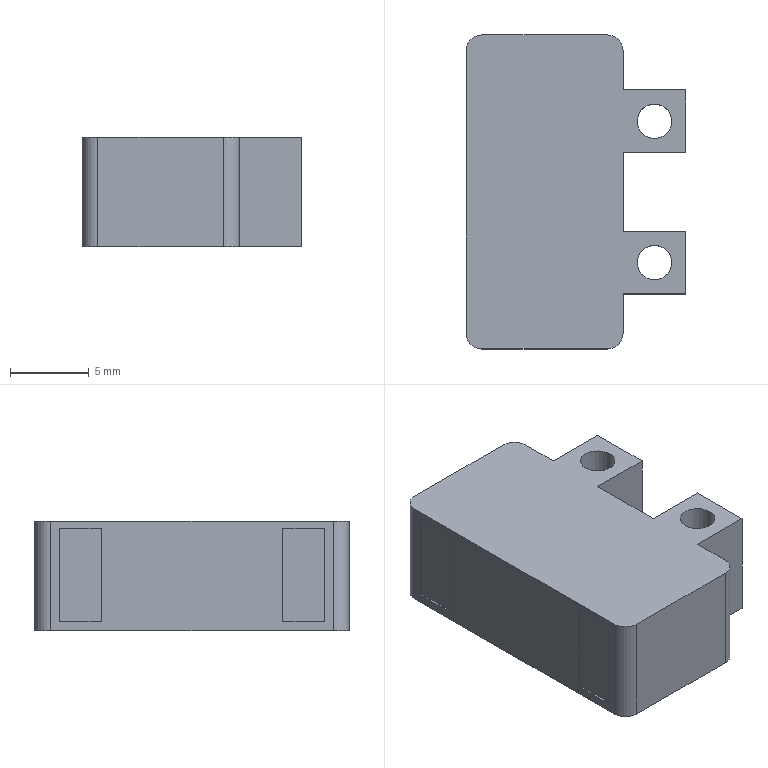Part | SolidWorks | features ICE 2, Extrusion 1, Fillet 1, MirrorPattern 1 | 1 solid | 32 faces | box 14 x 20 x 7 mm | volume 1562 mm3 | plane 24 | cylinder 8 | commonest cylinder face diameters 2 x4 2.2 x4
STEP:
#1=CARTESIAN_POINT('',(5.9,-4.5,0.));
#2=VERTEX_POINT('',#1);
#3=CARTESIAN_POINT('',(8.1,-4.5,0.));
#4=VERTEX_POINT('',#3);
#5=CARTESIAN_POINT('',(7.,-4.5,0.));
#6=DIRECTION('',(0.,0.,1.));
#7=DIRECTION('',(1.,0.,0.));
#8=AXIS2_PLACEMENT_3D('',#5,#6,#7);
#9=CIRCLE('',#8,1.1);
#10=EDGE_CURVE('',#2,#4,#9,.T.);
#11=ORIENTED_EDGE('',*,*,#10,.F.);
#12=CARTESIAN_POINT('',(5.9,-4.5,7.));
#13=VERTEX_POINT('',#12);
#14=CARTESIAN_POINT('',(5.9,-4.5,0.));
#15=DIRECTION('',(0.,0.,1.));
#16=VECTOR('',#15,1000.);
#17=LINE('',#14,#16);
#18=EDGE_CURVE('',#2,#13,#17,.T.);
#19=ORIENTED_EDGE('',*,*,#18,.T.);
#20=CARTESIAN_POINT('',(8.1,-4.5,7.));
#21=VERTEX_POINT('',#20);
#22=CARTESIAN_POINT('',(7.,-4.5,7.));
#23=DIRECTION('',(0.,0.,1.));
#24=DIRECTION('',(1.,0.,0.));
#25=AXIS2_PLACEMENT_3D('',#22,#23,#24);
#26=CIRCLE('',#25,1.1);
#27=EDGE_CURVE('',#13,#21,#26,.T.);
#28=ORIENTED_EDGE('',*,*,#27,.T.);
#29=CARTESIAN_POINT('',(8.1,-4.5,0.));
#30=DIRECTION('',(0.,0.,1.));
#31=VECTOR('',#30,1000.);
#32=LINE('',#29,#31);
#33=EDGE_CURVE('',#4,#21,#32,.T.);
#34=ORIENTED_EDGE('',*,*,#33,.F.);
#35=EDGE_LOOP('',(#11,#19,#28,#34));
#36=FACE_OUTER_BOUND('',#35,.T.);
#37=CARTESIAN_POINT('',(7.,-4.5,0.));
#38=DIRECTION('',(0.,0.,1.));
#39=DIRECTION('',(1.,0.,0.));
#40=AXIS2_PLACEMENT_3D('',#37,#38,#39);
#41=CYLINDRICAL_SURFACE('',#40,1.1);
#42=ADVANCED_FACE('',(#36),#41,.F.);
#43=CARTESIAN_POINT('',(5.9,4.5,0.));
#44=VERTEX_POINT('',#43);
#45=CARTESIAN_POINT('',(8.1,4.5,0.));
#46=VERTEX_POINT('',#45);
#47=CARTESIAN_POINT('',(7.,4.5,0.));
#48=DIRECTION('',(0.,0.,1.));
#49=DIRECTION('',(1.,0.,0.));
#50=AXIS2_PLACEMENT_3D('',#47,#48,#49);
#51=CIRCLE('',#50,1.1);
#52=EDGE_CURVE('',#44,#46,#51,.T.);
#53=ORIENTED_EDGE('',*,*,#52,.F.);
#54=CARTESIAN_POINT('',(5.9,4.5,7.));
#55=VERTEX_POINT('',#54);
#56=CARTESIAN_POINT('',(5.9,4.5,0.));
#57=DIRECTION('',(0.,0.,1.));
#58=VECTOR('',#57,1000.);
#59=LINE('',#56,#58);
#60=EDGE_CURVE('',#44,#55,#59,.T.);
#61=ORIENTED_EDGE('',*,*,#60,.T.);
#62=CARTESIAN_POINT('',(8.1,4.5,7.));
#63=VERTEX_POINT('',#62);
#64=CARTESIAN_POINT('',(7.,4.5,7.));
#65=DIRECTION('',(0.,0.,1.));
#66=DIRECTION('',(1.,0.,0.));
#67=AXIS2_PLACEMENT_3D('',#64,#65,#66);
#68=CIRCLE('',#67,1.1);
#69=EDGE_CURVE('',#55,#63,#68,.T.);
#70=ORIENTED_EDGE('',*,*,#69,.T.);
#71=CARTESIAN_POINT('',(8.1,4.5,0.));
#72=DIRECTION('',(0.,0.,1.));
#73=VECTOR('',#72,1000.);
#74=LINE('',#71,#73);
#75=EDGE_CURVE('',#46,#63,#74,.T.);
#76=ORIENTED_EDGE('',*,*,#75,.F.);
#77=EDGE_LOOP('',(#53,#61,#70,#76));
#78=FACE_OUTER_BOUND('',#77,.T.);
#79=CARTESIAN_POINT('',(7.,4.5,0.));
#80=DIRECTION('',(0.,0.,1.));
#81=DIRECTION('',(1.,0.,0.));
#82=AXIS2_PLACEMENT_3D('',#79,#80,#81);
#83=CYLINDRICAL_SURFACE('',#82,1.1);
#84=ADVANCED_FACE('',(#78),#83,.F.);
#85=CARTESIAN_POINT('',(-5.,9.,0.));
#86=VERTEX_POINT('',#85);
#87=CARTESIAN_POINT('',(-5.,-9.,0.));
#88=VERTEX_POINT('',#87);
#89=CARTESIAN_POINT('',(-5.,10.,0.));
#90=DIRECTION('',(0.,-1.,0.));
#91=VECTOR('',#90,1000.);
#92=LINE('',#89,#91);
#93=EDGE_CURVE('',#86,#88,#92,.T.);
#94=ORIENTED_EDGE('',*,*,#93,.T.);
#95=CARTESIAN_POINT('',(-5.,-9.,7.));
#96=VERTEX_POINT('',#95);
#97=CARTESIAN_POINT('',(-5.,-9.,7.));
#98=DIRECTION('',(0.,0.,1.));
#99=VECTOR('',#98,1000.);
#100=LINE('',#97,#99);
#101=EDGE_CURVE('',#88,#96,#100,.T.);
#102=ORIENTED_EDGE('',*,*,#101,.T.);
#103=CARTESIAN_POINT('',(-5.,9.,7.));
#104=VERTEX_POINT('',#103);
#105=CARTESIAN_POINT('',(-5.,10.,7.));
#106=DIRECTION('',(0.,-1.,0.));
#107=VECTOR('',#106,1000.);
#108=LINE('',#105,#107);
#109=EDGE_CURVE('',#104,#96,#108,.T.);
#110=ORIENTED_EDGE('',*,*,#109,.F.);
#111=CARTESIAN_POINT('',(-5.,9.,7.));
#112=DIRECTION('',(0.,0.,-1.));
#113=VECTOR('',#112,1000.);
#114=LINE('',#111,#113);
#115=EDGE_CURVE('',#104,#86,#114,.T.);
#116=ORIENTED_EDGE('',*,*,#115,.T.);
#117=EDGE_LOOP('',(#94,#102,#110,#116));
#118=FACE_OUTER_BOUND('',#117,.T.);
#119=CARTESIAN_POINT('',(-5.,5.784,0.5738));
#120=VERTEX_POINT('',#119);
#121=CARTESIAN_POINT('',(-5.,5.784,6.528));
#122=VERTEX_POINT('',#121);
#123=CARTESIAN_POINT('',(-5.,5.784,0.5738));
#124=DIRECTION('',(0.,0.,1.));
#125=VECTOR('',#124,1000.);
#126=LINE('',#123,#125);
#127=EDGE_CURVE('',#120,#122,#126,.T.);
#128=ORIENTED_EDGE('',*,*,#127,.F.);
#129=CARTESIAN_POINT('',(-5.,8.438,0.5738));
#130=VERTEX_POINT('',#129);
#131=CARTESIAN_POINT('',(-5.,8.438,0.5738));
#132=DIRECTION('',(0.,-1.,0.));
#133=VECTOR('',#132,1000.);
#134=LINE('',#131,#133);
#135=EDGE_CURVE('',#130,#120,#134,.T.);
#136=ORIENTED_EDGE('',*,*,#135,.F.);
#137=CARTESIAN_POINT('',(-5.,8.438,6.528));
#138=VERTEX_POINT('',#137);
#139=CARTESIAN_POINT('',(-5.,8.438,0.5738));
#140=DIRECTION('',(0.,0.,-1.));
#141=VECTOR('',#140,1000.);
#142=LINE('',#139,#141);
#143=EDGE_CURVE('',#138,#130,#142,.T.);
#144=ORIENTED_EDGE('',*,*,#143,.F.);
#145=CARTESIAN_POINT('',(-5.,8.438,6.528));
#146=DIRECTION('',(0.,1.,0.));
#147=VECTOR('',#146,1000.);
#148=LINE('',#145,#147);
#149=EDGE_CURVE('',#122,#138,#148,.T.);
#150=ORIENTED_EDGE('',*,*,#149,.F.);
#151=EDGE_LOOP('',(#128,#136,#144,#150));
#152=FACE_BOUND('',#151,.T.);
#153=CARTESIAN_POINT('',(-5.,-8.438,0.5738));
#154=VERTEX_POINT('',#153);
#155=CARTESIAN_POINT('',(-5.,-5.784,0.5738));
#156=VERTEX_POINT('',#155);
#157=CARTESIAN_POINT('',(-5.,-8.438,0.5738));
#158=DIRECTION('',(0.,1.,0.));
#159=VECTOR('',#158,1000.);
#160=LINE('',#157,#159);
#161=EDGE_CURVE('',#154,#156,#160,.T.);
#162=ORIENTED_EDGE('',*,*,#161,.T.);
#163=CARTESIAN_POINT('',(-5.,-5.784,6.528));
#164=VERTEX_POINT('',#163);
#165=CARTESIAN_POINT('',(-5.,-5.784,0.5738));
#166=DIRECTION('',(0.,0.,1.));
#167=VECTOR('',#166,1000.);
#168=LINE('',#165,#167);
#169=EDGE_CURVE('',#156,#164,#168,.T.);
#170=ORIENTED_EDGE('',*,*,#169,.T.);
#171=CARTESIAN_POINT('',(-5.,-8.438,6.528));
#172=VERTEX_POINT('',#171);
#173=CARTESIAN_POINT('',(-5.,-8.438,6.528));
#174=DIRECTION('',(0.,-1.,0.));
#175=VECTOR('',#174,1000.);
#176=LINE('',#173,#175);
#177=EDGE_CURVE('',#164,#172,#176,.T.);
#178=ORIENTED_EDGE('',*,*,#177,.T.);
#179=CARTESIAN_POINT('',(-5.,-8.438,0.5738));
#180=DIRECTION('',(0.,0.,-1.));
#181=VECTOR('',#180,1000.);
#182=LINE('',#179,#181);
#183=EDGE_CURVE('',#172,#154,#182,.T.);
#184=ORIENTED_EDGE('',*,*,#183,.T.);
#185=EDGE_LOOP('',(#162,#170,#178,#184));
#186=FACE_BOUND('',#185,.T.);
#187=CARTESIAN_POINT('',(-5.,10.,7.));
#188=DIRECTION('',(1.,0.,0.));
#189=DIRECTION('',(0.,1.,0.));
#190=AXIS2_PLACEMENT_3D('',#187,#188,#189);
#191=PLANE('',#190);
#192=ADVANCED_FACE('',(#118,#152,#186),#191,.F.);
#193=CARTESIAN_POINT('',(5.,-2.5,7.));
#194=VERTEX_POINT('',#193);
#195=CARTESIAN_POINT('',(5.,2.5,7.));
#196=VERTEX_POINT('',#195);
#197=CARTESIAN_POINT('',(5.,10.,7.));
#198=DIRECTION('',(0.,1.,0.));
#199=VECTOR('',#198,1000.);
#200=LINE('',#197,#199);
#201=EDGE_CURVE('',#194,#196,#200,.T.);
#202=ORIENTED_EDGE('',*,*,#201,.F.);
#203=CARTESIAN_POINT('',(5.,-2.5,0.));
#204=VERTEX_POINT('',#203);
#205=CARTESIAN_POINT('',(5.,-2.5,0.));
#206=DIRECTION('',(0.,0.,1.));
#207=VECTOR('',#206,1000.);
#208=LINE('',#205,#207);
#209=EDGE_CURVE('',#204,#194,#208,.T.);
#210=ORIENTED_EDGE('',*,*,#209,.F.);
#211=CARTESIAN_POINT('',(5.,2.5,0.));
#212=VERTEX_POINT('',#211);
#213=CARTESIAN_POINT('',(5.,10.,0.));
#214=DIRECTION('',(0.,1.,0.));
#215=VECTOR('',#214,1000.);
#216=LINE('',#213,#215);
#217=EDGE_CURVE('',#204,#212,#216,.T.);
#218=ORIENTED_EDGE('',*,*,#217,.T.);
#219=CARTESIAN_POINT('',(5.,2.5,0.));
#220=DIRECTION('',(0.,0.,1.));
#221=VECTOR('',#220,1000.);
#222=LINE('',#219,#221);
#223=EDGE_CURVE('',#212,#196,#222,.T.);
#224=ORIENTED_EDGE('',*,*,#223,.T.);
#225=EDGE_LOOP('',(#202,#210,#218,#224));
#226=FACE_OUTER_BOUND('',#225,.T.);
#227=CARTESIAN_POINT('',(5.,10.,7.));
#228=DIRECTION('',(-1.,0.,0.));
#229=DIRECTION('',(0.,-1.,0.));
#230=AXIS2_PLACEMENT_3D('',#227,#228,#229);
#231=PLANE('',#230);
#232=ADVANCED_FACE('',(#226),#231,.F.);
#233=CARTESIAN_POINT('',(5.,6.5,0.));
#234=VERTEX_POINT('',#233);
#235=CARTESIAN_POINT('',(5.,9.,0.));
#236=VERTEX_POINT('',#235);
#237=CARTESIAN_POINT('',(5.,10.,0.));
#238=DIRECTION('',(0.,1.,0.));
#239=VECTOR('',#238,1000.);
#240=LINE('',#237,#239);
#241=EDGE_CURVE('',#234,#236,#240,.T.);
#242=ORIENTED_EDGE('',*,*,#241,.T.);
#243=CARTESIAN_POINT('',(5.,9.,7.));
#244=VERTEX_POINT('',#243);
#245=CARTESIAN_POINT('',(5.,9.,7.));
#246=DIRECTION('',(0.,0.,1.));
#247=VECTOR('',#246,1000.);
#248=LINE('',#245,#247);
#249=EDGE_CURVE('',#236,#244,#248,.T.);
#250=ORIENTED_EDGE('',*,*,#249,.T.);
#251=CARTESIAN_POINT('',(5.,6.5,7.));
#252=VERTEX_POINT('',#251);
#253=CARTESIAN_POINT('',(5.,10.,7.));
#254=DIRECTION('',(0.,1.,0.));
#255=VECTOR('',#254,1000.);
#256=LINE('',#253,#255);
#257=EDGE_CURVE('',#252,#244,#256,.T.);
#258=ORIENTED_EDGE('',*,*,#257,.F.);
#259=CARTESIAN_POINT('',(5.,6.5,0.));
#260=DIRECTION('',(0.,0.,1.));
#261=VECTOR('',#260,1000.);
#262=LINE('',#259,#261);
#263=EDGE_CURVE('',#234,#252,#262,.T.);
#264=ORIENTED_EDGE('',*,*,#263,.F.);
#265=EDGE_LOOP('',(#242,#250,#258,#264));
#266=FACE_OUTER_BOUND('',#265,.T.);
#267=CARTESIAN_POINT('',(5.,10.,7.));
#268=DIRECTION('',(-1.,0.,0.));
#269=DIRECTION('',(0.,-1.,0.));
#270=AXIS2_PLACEMENT_3D('',#267,#268,#269);
#271=PLANE('',#270);
#272=ADVANCED_FACE('',(#266),#271,.F.);
#273=CARTESIAN_POINT('',(5.,-9.,7.));
#274=VERTEX_POINT('',#273);
#275=CARTESIAN_POINT('',(5.,-6.5,7.));
#276=VERTEX_POINT('',#275);
#277=CARTESIAN_POINT('',(5.,10.,7.));
#278=DIRECTION('',(0.,1.,0.));
#279=VECTOR('',#278,1000.);
#280=LINE('',#277,#279);
#281=EDGE_CURVE('',#274,#276,#280,.T.);
#282=ORIENTED_EDGE('',*,*,#281,.F.);
#283=CARTESIAN_POINT('',(5.,-9.,0.));
#284=VERTEX_POINT('',#283);
#285=CARTESIAN_POINT('',(5.,-9.,7.));
#286=DIRECTION('',(0.,0.,-1.));
#287=VECTOR('',#286,1000.);
#288=LINE('',#285,#287);
#289=EDGE_CURVE('',#274,#284,#288,.T.);
#290=ORIENTED_EDGE('',*,*,#289,.T.);
#291=CARTESIAN_POINT('',(5.,-6.5,0.));
#292=VERTEX_POINT('',#291);
#293=CARTESIAN_POINT('',(5.,10.,0.));
#294=DIRECTION('',(0.,1.,0.));
#295=VECTOR('',#294,1000.);
#296=LINE('',#293,#295);
#297=EDGE_CURVE('',#284,#292,#296,.T.);
#298=ORIENTED_EDGE('',*,*,#297,.T.);
#299=CARTESIAN_POINT('',(5.,-6.5,0.));
#300=DIRECTION('',(0.,0.,1.));
#301=VECTOR('',#300,1000.);
#302=LINE('',#299,#301);
#303=EDGE_CURVE('',#292,#276,#302,.T.);
#304=ORIENTED_EDGE('',*,*,#303,.T.);
#305=EDGE_LOOP('',(#282,#290,#298,#304));
#306=FACE_OUTER_BOUND('',#305,.T.);
#307=CARTESIAN_POINT('',(5.,10.,7.));
#308=DIRECTION('',(-1.,0.,0.));
#309=DIRECTION('',(0.,-1.,0.));
#310=AXIS2_PLACEMENT_3D('',#307,#308,#309);
#311=PLANE('',#310);
#312=ADVANCED_FACE('',(#306),#311,.F.);
#313=CARTESIAN_POINT('',(4.,10.,7.));
#314=VERTEX_POINT('',#313);
#315=CARTESIAN_POINT('',(-4.,10.,7.));
#316=VERTEX_POINT('',#315);
#317=CARTESIAN_POINT('',(-5.,10.,7.));
#318=DIRECTION('',(-1.,0.,0.));
#319=VECTOR('',#318,1000.);
#320=LINE('',#317,#319);
#321=EDGE_CURVE('',#314,#316,#320,.T.);
#322=ORIENTED_EDGE('',*,*,#321,.F.);
#323=CARTESIAN_POINT('',(4.,10.,0.));
#324=VERTEX_POINT('',#323);
#325=CARTESIAN_POINT('',(4.,10.,7.));
#326=DIRECTION('',(0.,0.,-1.));
#327=VECTOR('',#326,1000.);
#328=LINE('',#325,#327);
#329=EDGE_CURVE('',#314,#324,#328,.T.);
#330=ORIENTED_EDGE('',*,*,#329,.T.);
#331=CARTESIAN_POINT('',(-4.,10.,0.));
#332=VERTEX_POINT('',#331);
#333=CARTESIAN_POINT('',(-5.,10.,0.));
#334=DIRECTION('',(-1.,0.,0.));
#335=VECTOR('',#334,1000.);
#336=LINE('',#333,#335);
#337=EDGE_CURVE('',#324,#332,#336,.T.);
#338=ORIENTED_EDGE('',*,*,#337,.T.);
#339=CARTESIAN_POINT('',(-4.,10.,7.));
#340=DIRECTION('',(0.,0.,1.));
#341=VECTOR('',#340,1000.);
#342=LINE('',#339,#341);
#343=EDGE_CURVE('',#332,#316,#342,.T.);
#344=ORIENTED_EDGE('',*,*,#343,.T.);
#345=EDGE_LOOP('',(#322,#330,#338,#344));
#346=FACE_OUTER_BOUND('',#345,.T.);
#347=CARTESIAN_POINT('',(-5.,10.,7.));
#348=DIRECTION('',(0.,-1.,0.));
#349=DIRECTION('',(0.,0.,-1.));
#350=AXIS2_PLACEMENT_3D('',#347,#348,#349);
#351=PLANE('',#350);
#352=ADVANCED_FACE('',(#346),#351,.F.);
#353=CARTESIAN_POINT('',(-4.,-10.,0.));
#354=VERTEX_POINT('',#353);
#355=CARTESIAN_POINT('',(4.,-10.,0.));
#356=VERTEX_POINT('',#355);
#357=CARTESIAN_POINT('',(-5.,-10.,0.));
#358=DIRECTION('',(1.,0.,0.));
#359=VECTOR('',#358,1000.);
#360=LINE('',#357,#359);
#361=EDGE_CURVE('',#354,#356,#360,.T.);
#362=ORIENTED_EDGE('',*,*,#361,.T.);
#363=CARTESIAN_POINT('',(4.,-10.,7.));
#364=VERTEX_POINT('',#363);
#365=CARTESIAN_POINT('',(4.,-10.,7.));
#366=DIRECTION('',(0.,0.,1.));
#367=VECTOR('',#366,1000.);
#368=LINE('',#365,#367);
#369=EDGE_CURVE('',#356,#364,#368,.T.);
#370=ORIENTED_EDGE('',*,*,#369,.T.);
#371=CARTESIAN_POINT('',(-4.,-10.,7.));
#372=VERTEX_POINT('',#371);
#373=CARTESIAN_POINT('',(-5.,-10.,7.));
#374=DIRECTION('',(1.,0.,0.));
#375=VECTOR('',#374,1000.);
#376=LINE('',#373,#375);
#377=EDGE_CURVE('',#372,#364,#376,.T.);
#378=ORIENTED_EDGE('',*,*,#377,.F.);
#379=CARTESIAN_POINT('',(-4.,-10.,7.));
#380=DIRECTION('',(0.,0.,-1.));
#381=VECTOR('',#380,1000.);
#382=LINE('',#379,#381);
#383=EDGE_CURVE('',#372,#354,#382,.T.);
#384=ORIENTED_EDGE('',*,*,#383,.T.);
#385=EDGE_LOOP('',(#362,#370,#378,#384));
#386=FACE_OUTER_BOUND('',#385,.T.);
#387=CARTESIAN_POINT('',(-5.,-10.,7.));
#388=DIRECTION('',(0.,1.,0.));
#389=DIRECTION('',(0.,0.,1.));
#390=AXIS2_PLACEMENT_3D('',#387,#388,#389);
#391=PLANE('',#390);
#392=ADVANCED_FACE('',(#386),#391,.F.);
#393=ORIENTED_EDGE('',*,*,#377,.T.);
#394=CARTESIAN_POINT('',(4.,-9.,7.));
#395=DIRECTION('',(0.,0.,1.));
#396=DIRECTION('',(1.,0.,0.));
#397=AXIS2_PLACEMENT_3D('',#394,#395,#396);
#398=CIRCLE('',#397,1.);
#399=EDGE_CURVE('',#364,#274,#398,.T.);
#400=ORIENTED_EDGE('',*,*,#399,.T.);
#401=ORIENTED_EDGE('',*,*,#281,.T.);
#402=CARTESIAN_POINT('',(9.,-6.5,7.));
#403=VERTEX_POINT('',#402);
#404=CARTESIAN_POINT('',(5.,-6.5,7.));
#405=DIRECTION('',(1.,0.,0.));
#406=VECTOR('',#405,1000.);
#407=LINE('',#404,#406);
#408=EDGE_CURVE('',#276,#403,#407,.T.);
#409=ORIENTED_EDGE('',*,*,#408,.T.);
#410=CARTESIAN_POINT('',(9.,-2.5,7.));
#411=VERTEX_POINT('',#410);
#412=CARTESIAN_POINT('',(9.,-2.5,7.));
#413=DIRECTION('',(0.,1.,0.));
#414=VECTOR('',#413,1000.);
#415=LINE('',#412,#414);
#416=EDGE_CURVE('',#403,#411,#415,.T.);
#417=ORIENTED_EDGE('',*,*,#416,.T.);
#418=CARTESIAN_POINT('',(5.,-2.5,7.));
#419=DIRECTION('',(-1.,0.,0.));
#420=VECTOR('',#419,1000.);
#421=LINE('',#418,#420);
#422=EDGE_CURVE('',#411,#194,#421,.T.);
#423=ORIENTED_EDGE('',*,*,#422,.T.);
#424=ORIENTED_EDGE('',*,*,#201,.T.);
#425=CARTESIAN_POINT('',(9.,2.5,7.));
#426=VERTEX_POINT('',#425);
#427=CARTESIAN_POINT('',(5.,2.5,7.));
#428=DIRECTION('',(1.,0.,0.));
#429=VECTOR('',#428,1000.);
#430=LINE('',#427,#429);
#431=EDGE_CURVE('',#196,#426,#430,.T.);
#432=ORIENTED_EDGE('',*,*,#431,.T.);
#433=CARTESIAN_POINT('',(9.,6.5,7.));
#434=VERTEX_POINT('',#433);
#435=CARTESIAN_POINT('',(9.,6.5,7.));
#436=DIRECTION('',(0.,1.,0.));
#437=VECTOR('',#436,1000.);
#438=LINE('',#435,#437);
#439=EDGE_CURVE('',#426,#434,#438,.T.);
#440=ORIENTED_EDGE('',*,*,#439,.T.);
#441=CARTESIAN_POINT('',(5.,6.5,7.));
#442=DIRECTION('',(-1.,0.,0.));
#443=VECTOR('',#442,1000.);
#444=LINE('',#441,#443);
#445=EDGE_CURVE('',#434,#252,#444,.T.);
#446=ORIENTED_EDGE('',*,*,#445,.T.);
#447=ORIENTED_EDGE('',*,*,#257,.T.);
#448=CARTESIAN_POINT('',(4.,9.,7.));
#449=DIRECTION('',(0.,0.,1.));
#450=DIRECTION('',(1.,0.,0.));
#451=AXIS2_PLACEMENT_3D('',#448,#449,#450);
#452=CIRCLE('',#451,1.);
#453=EDGE_CURVE('',#244,#314,#452,.T.);
#454=ORIENTED_EDGE('',*,*,#453,.T.);
#455=ORIENTED_EDGE('',*,*,#321,.T.);
#456=CARTESIAN_POINT('',(-4.,9.,7.));
#457=DIRECTION('',(0.,0.,1.));
#458=DIRECTION('',(1.,0.,0.));
#459=AXIS2_PLACEMENT_3D('',#456,#457,#458);
#460=CIRCLE('',#459,1.);
#461=EDGE_CURVE('',#316,#104,#460,.T.);
#462=ORIENTED_EDGE('',*,*,#461,.T.);
#463=ORIENTED_EDGE('',*,*,#109,.T.);
#464=CARTESIAN_POINT('',(-4.,-9.,7.));
#465=DIRECTION('',(0.,0.,1.));
#466=DIRECTION('',(1.,0.,0.));
#467=AXIS2_PLACEMENT_3D('',#464,#465,#466);
#468=CIRCLE('',#467,1.);
#469=EDGE_CURVE('',#96,#372,#468,.T.);
#470=ORIENTED_EDGE('',*,*,#469,.T.);
#471=EDGE_LOOP('',(#393,#400,#401,#409,#417,#423,#424,#432,#440,#446,#447,#454,#455,#462,#463,#470));
#472=FACE_OUTER_BOUND('',#471,.T.);
#473=CARTESIAN_POINT('',(7.,4.5,7.));
#474=DIRECTION('',(0.,0.,1.));
#475=DIRECTION('',(1.,0.,0.));
#476=AXIS2_PLACEMENT_3D('',#473,#474,#475);
#477=CIRCLE('',#476,1.1);
#478=EDGE_CURVE('',#63,#55,#477,.T.);
#479=ORIENTED_EDGE('',*,*,#478,.F.);
#480=ORIENTED_EDGE('',*,*,#69,.F.);
#481=EDGE_LOOP('',(#479,#480));
#482=FACE_BOUND('',#481,.T.);
#483=CARTESIAN_POINT('',(7.,-4.5,7.));
#484=DIRECTION('',(0.,0.,1.));
#485=DIRECTION('',(1.,0.,0.));
#486=AXIS2_PLACEMENT_3D('',#483,#484,#485);
#487=CIRCLE('',#486,1.1);
#488=EDGE_CURVE('',#21,#13,#487,.T.);
#489=ORIENTED_EDGE('',*,*,#488,.F.);
#490=ORIENTED_EDGE('',*,*,#27,.F.);
#491=EDGE_LOOP('',(#489,#490));
#492=FACE_BOUND('',#491,.T.);
#493=CARTESIAN_POINT('',(5.,-10.,7.));
#494=DIRECTION('',(0.,0.,1.));
#495=DIRECTION('',(1.,0.,0.));
#496=AXIS2_PLACEMENT_3D('',#493,#494,#495);
#497=PLANE('',#496);
#498=ADVANCED_FACE('',(#472,#482,#492),#497,.T.);
#499=ORIENTED_EDGE('',*,*,#297,.F.);
#500=CARTESIAN_POINT('',(4.,-9.,0.));
#501=DIRECTION('',(0.,0.,-1.));
#502=DIRECTION('',(1.,0.,0.));
#503=AXIS2_PLACEMENT_3D('',#500,#501,#502);
#504=CIRCLE('',#503,1.);
#505=EDGE_CURVE('',#284,#356,#504,.T.);
#506=ORIENTED_EDGE('',*,*,#505,.T.);
#507=ORIENTED_EDGE('',*,*,#361,.F.);
#508=CARTESIAN_POINT('',(-4.,-9.,0.));
#509=DIRECTION('',(0.,0.,-1.));
#510=DIRECTION('',(1.,0.,0.));
#511=AXIS2_PLACEMENT_3D('',#508,#509,#510);
#512=CIRCLE('',#511,1.);
#513=EDGE_CURVE('',#354,#88,#512,.T.);
#514=ORIENTED_EDGE('',*,*,#513,.T.);
#515=ORIENTED_EDGE('',*,*,#93,.F.);
#516=CARTESIAN_POINT('',(-4.,9.,0.));
#517=DIRECTION('',(0.,0.,-1.));
#518=DIRECTION('',(1.,0.,0.));
#519=AXIS2_PLACEMENT_3D('',#516,#517,#518);
#520=CIRCLE('',#519,1.);
#521=EDGE_CURVE('',#86,#332,#520,.T.);
#522=ORIENTED_EDGE('',*,*,#521,.T.);
#523=ORIENTED_EDGE('',*,*,#337,.F.);
#524=CARTESIAN_POINT('',(4.,9.,0.));
#525=DIRECTION('',(0.,0.,-1.));
#526=DIRECTION('',(1.,0.,0.));
#527=AXIS2_PLACEMENT_3D('',#524,#525,#526);
#528=CIRCLE('',#527,1.);
#529=EDGE_CURVE('',#324,#236,#528,.T.);
#530=ORIENTED_EDGE('',*,*,#529,.T.);
#531=ORIENTED_EDGE('',*,*,#241,.F.);
#532=CARTESIAN_POINT('',(9.,6.5,0.));
#533=VERTEX_POINT('',#532);
#534=CARTESIAN_POINT('',(5.,6.5,0.));
#535=DIRECTION('',(-1.,0.,0.));
#536=VECTOR('',#535,1000.);
#537=LINE('',#534,#536);
#538=EDGE_CURVE('',#533,#234,#537,.T.);
#539=ORIENTED_EDGE('',*,*,#538,.F.);
#540=CARTESIAN_POINT('',(9.,2.5,0.));
#541=VERTEX_POINT('',#540);
#542=CARTESIAN_POINT('',(9.,6.5,0.));
#543=DIRECTION('',(0.,1.,0.));
#544=VECTOR('',#543,1000.);
#545=LINE('',#542,#544);
#546=EDGE_CURVE('',#541,#533,#545,.T.);
#547=ORIENTED_EDGE('',*,*,#546,.F.);
#548=CARTESIAN_POINT('',(5.,2.5,0.));
#549=DIRECTION('',(1.,0.,0.));
#550=VECTOR('',#549,1000.);
#551=LINE('',#548,#550);
#552=EDGE_CURVE('',#212,#541,#551,.T.);
#553=ORIENTED_EDGE('',*,*,#552,.F.);
#554=ORIENTED_EDGE('',*,*,#217,.F.);
#555=CARTESIAN_POINT('',(9.,-2.5,0.));
#556=VERTEX_POINT('',#555);
#557=CARTESIAN_POINT('',(5.,-2.5,0.));
#558=DIRECTION('',(-1.,0.,0.));
#559=VECTOR('',#558,1000.);
#560=LINE('',#557,#559);
#561=EDGE_CURVE('',#556,#204,#560,.T.);
#562=ORIENTED_EDGE('',*,*,#561,.F.);
#563=CARTESIAN_POINT('',(9.,-6.5,0.));
#564=VERTEX_POINT('',#563);
#565=CARTESIAN_POINT('',(9.,-2.5,0.));
#566=DIRECTION('',(0.,1.,0.));
#567=VECTOR('',#566,1000.);
#568=LINE('',#565,#567);
#569=EDGE_CURVE('',#564,#556,#568,.T.);
#570=ORIENTED_EDGE('',*,*,#569,.F.);
#571=CARTESIAN_POINT('',(5.,-6.5,0.));
#572=DIRECTION('',(1.,0.,0.));
#573=VECTOR('',#572,1000.);
#574=LINE('',#571,#573);
#575=EDGE_CURVE('',#292,#564,#574,.T.);
#576=ORIENTED_EDGE('',*,*,#575,.F.);
#577=EDGE_LOOP('',(#499,#506,#507,#514,#515,#522,#523,#530,#531,#539,#547,#553,#554,#562,#570,#576));
#578=FACE_OUTER_BOUND('',#577,.T.);
#579=CARTESIAN_POINT('',(7.,4.5,0.));
#580=DIRECTION('',(0.,0.,1.));
#581=DIRECTION('',(1.,0.,0.));
#582=AXIS2_PLACEMENT_3D('',#579,#580,#581);
#583=CIRCLE('',#582,1.1);
#584=EDGE_CURVE('',#46,#44,#583,.T.);
#585=ORIENTED_EDGE('',*,*,#584,.T.);
#586=ORIENTED_EDGE('',*,*,#52,.T.);
#587=EDGE_LOOP('',(#585,#586));
#588=FACE_BOUND('',#587,.T.);
#589=CARTESIAN_POINT('',(7.,-4.5,0.));
#590=DIRECTION('',(0.,0.,1.));
#591=DIRECTION('',(1.,0.,0.));
#592=AXIS2_PLACEMENT_3D('',#589,#590,#591);
#593=CIRCLE('',#592,1.1);
#594=EDGE_CURVE('',#4,#2,#593,.T.);
#595=ORIENTED_EDGE('',*,*,#594,.T.);
#596=ORIENTED_EDGE('',*,*,#10,.T.);
#597=EDGE_LOOP('',(#595,#596));
#598=FACE_BOUND('',#597,.T.);
#599=CARTESIAN_POINT('',(5.,-10.,0.));
#600=DIRECTION('',(0.,0.,1.));
#601=DIRECTION('',(1.,0.,0.));
#602=AXIS2_PLACEMENT_3D('',#599,#600,#601);
#603=PLANE('',#602);
#604=ADVANCED_FACE('',(#578,#588,#598),#603,.F.);
#605=ORIENTED_EDGE('',*,*,#445,.F.);
#606=CARTESIAN_POINT('',(9.,6.5,0.));
#607=DIRECTION('',(0.,0.,1.));
#608=VECTOR('',#607,1000.);
#609=LINE('',#606,#608);
#610=EDGE_CURVE('',#533,#434,#609,.T.);
#611=ORIENTED_EDGE('',*,*,#610,.F.);
#612=ORIENTED_EDGE('',*,*,#538,.T.);
#613=ORIENTED_EDGE('',*,*,#263,.T.);
#614=EDGE_LOOP('',(#605,#611,#612,#613));
#615=FACE_OUTER_BOUND('',#614,.T.);
#616=CARTESIAN_POINT('',(5.,6.5,0.));
#617=DIRECTION('',(0.,1.,0.));
#618=DIRECTION('',(0.,0.,1.));
#619=AXIS2_PLACEMENT_3D('',#616,#617,#618);
#620=PLANE('',#619);
#621=ADVANCED_FACE('',(#615),#620,.T.);
#622=ORIENTED_EDGE('',*,*,#439,.F.);
#623=CARTESIAN_POINT('',(9.,2.5,0.));
#624=DIRECTION('',(0.,0.,1.));
#625=VECTOR('',#624,1000.);
#626=LINE('',#623,#625);
#627=EDGE_CURVE('',#541,#426,#626,.T.);
#628=ORIENTED_EDGE('',*,*,#627,.F.);
#629=ORIENTED_EDGE('',*,*,#546,.T.);
#630=ORIENTED_EDGE('',*,*,#610,.T.);
#631=EDGE_LOOP('',(#622,#628,#629,#630));
#632=FACE_OUTER_BOUND('',#631,.T.);
#633=CARTESIAN_POINT('',(9.,6.5,0.));
#634=DIRECTION('',(1.,0.,0.));
#635=DIRECTION('',(0.,0.,-1.));
#636=AXIS2_PLACEMENT_3D('',#633,#634,#635);
#637=PLANE('',#636);
#638=ADVANCED_FACE('',(#632),#637,.T.);
#639=ORIENTED_EDGE('',*,*,#431,.F.);
#640=ORIENTED_EDGE('',*,*,#223,.F.);
#641=ORIENTED_EDGE('',*,*,#552,.T.);
#642=ORIENTED_EDGE('',*,*,#627,.T.);
#643=EDGE_LOOP('',(#639,#640,#641,#642));
#644=FACE_OUTER_BOUND('',#643,.T.);
#645=CARTESIAN_POINT('',(5.,2.5,0.));
#646=DIRECTION('',(0.,-1.,0.));
#647=DIRECTION('',(0.,0.,-1.));
#648=AXIS2_PLACEMENT_3D('',#645,#646,#647);
#649=PLANE('',#648);
#650=ADVANCED_FACE('',(#644),#649,.T.);
#651=ORIENTED_EDGE('',*,*,#60,.F.);
#652=ORIENTED_EDGE('',*,*,#584,.F.);
#653=ORIENTED_EDGE('',*,*,#75,.T.);
#654=ORIENTED_EDGE('',*,*,#478,.T.);
#655=EDGE_LOOP('',(#651,#652,#653,#654));
#656=FACE_OUTER_BOUND('',#655,.T.);
#657=CARTESIAN_POINT('',(7.,4.5,0.));
#658=DIRECTION('',(0.,0.,1.));
#659=DIRECTION('',(1.,0.,0.));
#660=AXIS2_PLACEMENT_3D('',#657,#658,#659);
#661=CYLINDRICAL_SURFACE('',#660,1.1);
#662=ADVANCED_FACE('',(#656),#661,.F.);
#663=ORIENTED_EDGE('',*,*,#422,.F.);
#664=CARTESIAN_POINT('',(9.,-2.5,0.));
#665=DIRECTION('',(0.,0.,1.));
#666=VECTOR('',#665,1000.);
#667=LINE('',#664,#666);
#668=EDGE_CURVE('',#556,#411,#667,.T.);
#669=ORIENTED_EDGE('',*,*,#668,.F.);
#670=ORIENTED_EDGE('',*,*,#561,.T.);
#671=ORIENTED_EDGE('',*,*,#209,.T.);
#672=EDGE_LOOP('',(#663,#669,#670,#671));
#673=FACE_OUTER_BOUND('',#672,.T.);
#674=CARTESIAN_POINT('',(5.,-2.5,0.));
#675=DIRECTION('',(0.,1.,0.));
#676=DIRECTION('',(0.,0.,1.));
#677=AXIS2_PLACEMENT_3D('',#674,#675,#676);
#678=PLANE('',#677);
#679=ADVANCED_FACE('',(#673),#678,.T.);
#680=ORIENTED_EDGE('',*,*,#416,.F.);
#681=CARTESIAN_POINT('',(9.,-6.5,0.));
#682=DIRECTION('',(0.,0.,1.));
#683=VECTOR('',#682,1000.);
#684=LINE('',#681,#683);
#685=EDGE_CURVE('',#564,#403,#684,.T.);
#686=ORIENTED_EDGE('',*,*,#685,.F.);
#687=ORIENTED_EDGE('',*,*,#569,.T.);
#688=ORIENTED_EDGE('',*,*,#668,.T.);
#689=EDGE_LOOP('',(#680,#686,#687,#688));
#690=FACE_OUTER_BOUND('',#689,.T.);
#691=CARTESIAN_POINT('',(9.,-2.5,0.));
#692=DIRECTION('',(1.,0.,0.));
#693=DIRECTION('',(0.,0.,-1.));
#694=AXIS2_PLACEMENT_3D('',#691,#692,#693);
#695=PLANE('',#694);
#696=ADVANCED_FACE('',(#690),#695,.T.);
#697=ORIENTED_EDGE('',*,*,#408,.F.);
#698=ORIENTED_EDGE('',*,*,#303,.F.);
#699=ORIENTED_EDGE('',*,*,#575,.T.);
#700=ORIENTED_EDGE('',*,*,#685,.T.);
#701=EDGE_LOOP('',(#697,#698,#699,#700));
#702=FACE_OUTER_BOUND('',#701,.T.);
#703=CARTESIAN_POINT('',(5.,-6.5,0.));
#704=DIRECTION('',(0.,-1.,0.));
#705=DIRECTION('',(0.,0.,-1.));
#706=AXIS2_PLACEMENT_3D('',#703,#704,#705);
#707=PLANE('',#706);
#708=ADVANCED_FACE('',(#702),#707,.T.);
#709=ORIENTED_EDGE('',*,*,#18,.F.);
#710=ORIENTED_EDGE('',*,*,#594,.F.);
#711=ORIENTED_EDGE('',*,*,#33,.T.);
#712=ORIENTED_EDGE('',*,*,#488,.T.);
#713=EDGE_LOOP('',(#709,#710,#711,#712));
#714=FACE_OUTER_BOUND('',#713,.T.);
#715=CARTESIAN_POINT('',(7.,-4.5,0.));
#716=DIRECTION('',(0.,0.,1.));
#717=DIRECTION('',(1.,0.,0.));
#718=AXIS2_PLACEMENT_3D('',#715,#716,#717);
#719=CYLINDRICAL_SURFACE('',#718,1.1);
#720=ADVANCED_FACE('',(#714),#719,.F.);
#721=ORIENTED_EDGE('',*,*,#399,.F.);
#722=ORIENTED_EDGE('',*,*,#369,.F.);
#723=ORIENTED_EDGE('',*,*,#505,.F.);
#724=ORIENTED_EDGE('',*,*,#289,.F.);
#725=EDGE_LOOP('',(#721,#722,#723,#724));
#726=FACE_OUTER_BOUND('',#725,.T.);
#727=CARTESIAN_POINT('',(4.,-9.,7.));
#728=DIRECTION('',(0.,0.,-1.));
#729=DIRECTION('',(-1.,0.,0.));
#730=AXIS2_PLACEMENT_3D('',#727,#728,#729);
#731=CYLINDRICAL_SURFACE('',#730,1.);
#732=ADVANCED_FACE('',(#726),#731,.T.);
#733=ORIENTED_EDGE('',*,*,#469,.F.);
#734=ORIENTED_EDGE('',*,*,#101,.F.);
#735=ORIENTED_EDGE('',*,*,#513,.F.);
#736=ORIENTED_EDGE('',*,*,#383,.F.);
#737=EDGE_LOOP('',(#733,#734,#735,#736));
#738=FACE_OUTER_BOUND('',#737,.T.);
#739=CARTESIAN_POINT('',(-4.,-9.,7.));
#740=DIRECTION('',(0.,0.,-1.));
#741=DIRECTION('',(-1.,0.,0.));
#742=AXIS2_PLACEMENT_3D('',#739,#740,#741);
#743=CYLINDRICAL_SURFACE('',#742,1.);
#744=ADVANCED_FACE('',(#738),#743,.T.);
#745=ORIENTED_EDGE('',*,*,#453,.F.);
#746=ORIENTED_EDGE('',*,*,#249,.F.);
#747=ORIENTED_EDGE('',*,*,#529,.F.);
#748=ORIENTED_EDGE('',*,*,#329,.F.);
#749=EDGE_LOOP('',(#745,#746,#747,#748));
#750=FACE_OUTER_BOUND('',#749,.T.);
#751=CARTESIAN_POINT('',(4.,9.,7.));
#752=DIRECTION('',(0.,0.,-1.));
#753=DIRECTION('',(-1.,0.,0.));
#754=AXIS2_PLACEMENT_3D('',#751,#752,#753);
#755=CYLINDRICAL_SURFACE('',#754,1.);
#756=ADVANCED_FACE('',(#750),#755,.T.);
#757=ORIENTED_EDGE('',*,*,#461,.F.);
#758=ORIENTED_EDGE('',*,*,#343,.F.);
#759=ORIENTED_EDGE('',*,*,#521,.F.);
#760=ORIENTED_EDGE('',*,*,#115,.F.);
#761=EDGE_LOOP('',(#757,#758,#759,#760));
#762=FACE_OUTER_BOUND('',#761,.T.);
#763=CARTESIAN_POINT('',(-4.,9.,7.));
#764=DIRECTION('',(0.,0.,-1.));
#765=DIRECTION('',(-1.,0.,0.));
#766=AXIS2_PLACEMENT_3D('',#763,#764,#765);
#767=CYLINDRICAL_SURFACE('',#766,1.);
#768=ADVANCED_FACE('',(#762),#767,.T.);
#769=ORIENTED_EDGE('',*,*,#135,.T.);
#770=CARTESIAN_POINT('',(-4.9,5.784,0.5738));
#771=VERTEX_POINT('',#770);
#772=CARTESIAN_POINT('',(-4.9,5.784,0.5738));
#773=DIRECTION('',(-1.,0.,0.));
#774=VECTOR('',#773,1000.);
#775=LINE('',#772,#774);
#776=EDGE_CURVE('',#771,#120,#775,.T.);
#777=ORIENTED_EDGE('',*,*,#776,.F.);
#778=CARTESIAN_POINT('',(-4.9,8.438,0.5738));
#779=VERTEX_POINT('',#778);
#780=CARTESIAN_POINT('',(-4.9,8.438,0.5738));
#781=DIRECTION('',(0.,-1.,0.));
#782=VECTOR('',#781,1000.);
#783=LINE('',#780,#782);
#784=EDGE_CURVE('',#779,#771,#783,.T.);
#785=ORIENTED_EDGE('',*,*,#784,.F.);
#786=CARTESIAN_POINT('',(-4.9,8.438,0.5738));
#787=DIRECTION('',(-1.,0.,0.));
#788=VECTOR('',#787,1000.);
#789=LINE('',#786,#788);
#790=EDGE_CURVE('',#779,#130,#789,.T.);
#791=ORIENTED_EDGE('',*,*,#790,.T.);
#792=EDGE_LOOP('',(#769,#777,#785,#791));
#793=FACE_OUTER_BOUND('',#792,.T.);
#794=CARTESIAN_POINT('',(-4.9,8.438,0.5738));
#795=DIRECTION('',(0.,0.,-1.));
#796=DIRECTION('',(-1.,0.,0.));
#797=AXIS2_PLACEMENT_3D('',#794,#795,#796);
#798=PLANE('',#797);
#799=ADVANCED_FACE('',(#793),#798,.F.);
#800=ORIENTED_EDGE('',*,*,#143,.T.);
#801=ORIENTED_EDGE('',*,*,#790,.F.);
#802=CARTESIAN_POINT('',(-4.9,8.438,6.528));
#803=VERTEX_POINT('',#802);
#804=CARTESIAN_POINT('',(-4.9,8.438,0.5738));
#805=DIRECTION('',(0.,0.,-1.));
#806=VECTOR('',#805,1000.);
#807=LINE('',#804,#806);
#808=EDGE_CURVE('',#803,#779,#807,.T.);
#809=ORIENTED_EDGE('',*,*,#808,.F.);
#810=CARTESIAN_POINT('',(-4.9,8.438,6.528));
#811=DIRECTION('',(-1.,0.,0.));
#812=VECTOR('',#811,1000.);
#813=LINE('',#810,#812);
#814=EDGE_CURVE('',#803,#138,#813,.T.);
#815=ORIENTED_EDGE('',*,*,#814,.T.);
#816=EDGE_LOOP('',(#800,#801,#809,#815));
#817=FACE_OUTER_BOUND('',#816,.T.);
#818=CARTESIAN_POINT('',(-4.9,8.438,0.5738));
#819=DIRECTION('',(0.,1.,0.));
#820=DIRECTION('',(-1.,0.,0.));
#821=AXIS2_PLACEMENT_3D('',#818,#819,#820);
#822=PLANE('',#821);
#823=ADVANCED_FACE('',(#817),#822,.F.);
#824=ORIENTED_EDGE('',*,*,#149,.T.);
#825=ORIENTED_EDGE('',*,*,#814,.F.);
#826=CARTESIAN_POINT('',(-4.9,5.784,6.528));
#827=VERTEX_POINT('',#826);
#828=CARTESIAN_POINT('',(-4.9,8.438,6.528));
#829=DIRECTION('',(0.,1.,0.));
#830=VECTOR('',#829,1000.);
#831=LINE('',#828,#830);
#832=EDGE_CURVE('',#827,#803,#831,.T.);
#833=ORIENTED_EDGE('',*,*,#832,.F.);
#834=CARTESIAN_POINT('',(-4.9,5.784,6.528));
#835=DIRECTION('',(-1.,0.,0.));
#836=VECTOR('',#835,1000.);
#837=LINE('',#834,#836);
#838=EDGE_CURVE('',#827,#122,#837,.T.);
#839=ORIENTED_EDGE('',*,*,#838,.T.);
#840=EDGE_LOOP('',(#824,#825,#833,#839));
#841=FACE_OUTER_BOUND('',#840,.T.);
#842=CARTESIAN_POINT('',(-4.9,8.438,6.528));
#843=DIRECTION('',(0.,0.,1.));
#844=DIRECTION('',(1.,0.,0.));
#845=AXIS2_PLACEMENT_3D('',#842,#843,#844);
#846=PLANE('',#845);
#847=ADVANCED_FACE('',(#841),#846,.F.);
#848=ORIENTED_EDGE('',*,*,#127,.T.);
#849=ORIENTED_EDGE('',*,*,#838,.F.);
#850=CARTESIAN_POINT('',(-4.9,5.784,0.5738));
#851=DIRECTION('',(0.,0.,1.));
#852=VECTOR('',#851,1000.);
#853=LINE('',#850,#852);
#854=EDGE_CURVE('',#771,#827,#853,.T.);
#855=ORIENTED_EDGE('',*,*,#854,.F.);
#856=ORIENTED_EDGE('',*,*,#776,.T.);
#857=EDGE_LOOP('',(#848,#849,#855,#856));
#858=FACE_OUTER_BOUND('',#857,.T.);
#859=CARTESIAN_POINT('',(-4.9,5.784,0.5738));
#860=DIRECTION('',(0.,-1.,0.));
#861=DIRECTION('',(1.,0.,0.));
#862=AXIS2_PLACEMENT_3D('',#859,#860,#861);
#863=PLANE('',#862);
#864=ADVANCED_FACE('',(#858),#863,.F.);
#865=ORIENTED_EDGE('',*,*,#784,.T.);
#866=ORIENTED_EDGE('',*,*,#854,.T.);
#867=ORIENTED_EDGE('',*,*,#832,.T.);
#868=ORIENTED_EDGE('',*,*,#808,.T.);
#869=EDGE_LOOP('',(#865,#866,#867,#868));
#870=FACE_OUTER_BOUND('',#869,.T.);
#871=CARTESIAN_POINT('',(-4.9,5.784,0.5738));
#872=DIRECTION('',(-1.,0.,0.));
#873=DIRECTION('',(0.,0.,1.));
#874=AXIS2_PLACEMENT_3D('',#871,#872,#873);
#875=PLANE('',#874);
#876=ADVANCED_FACE('',(#870),#875,.T.);
#877=ORIENTED_EDGE('',*,*,#161,.F.);
#878=CARTESIAN_POINT('',(-4.9,-8.438,0.5738));
#879=VERTEX_POINT('',#878);
#880=CARTESIAN_POINT('',(-4.9,-8.438,0.5738));
#881=DIRECTION('',(-1.,0.,0.));
#882=VECTOR('',#881,1000.);
#883=LINE('',#880,#882);
#884=EDGE_CURVE('',#879,#154,#883,.T.);
#885=ORIENTED_EDGE('',*,*,#884,.F.);
#886=CARTESIAN_POINT('',(-4.9,-5.784,0.5738));
#887=VERTEX_POINT('',#886);
#888=CARTESIAN_POINT('',(-4.9,-8.438,0.5738));
#889=DIRECTION('',(0.,1.,0.));
#890=VECTOR('',#889,1000.);
#891=LINE('',#888,#890);
#892=EDGE_CURVE('',#879,#887,#891,.T.);
#893=ORIENTED_EDGE('',*,*,#892,.T.);
#894=CARTESIAN_POINT('',(-4.9,-5.784,0.5738));
#895=DIRECTION('',(-1.,0.,0.));
#896=VECTOR('',#895,1000.);
#897=LINE('',#894,#896);
#898=EDGE_CURVE('',#887,#156,#897,.T.);
#899=ORIENTED_EDGE('',*,*,#898,.T.);
#900=EDGE_LOOP('',(#877,#885,#893,#899));
#901=FACE_OUTER_BOUND('',#900,.T.);
#902=CARTESIAN_POINT('',(-4.9,-8.438,0.5738));
#903=DIRECTION('',(0.,0.,1.));
#904=DIRECTION('',(1.,0.,0.));
#905=AXIS2_PLACEMENT_3D('',#902,#903,#904);
#906=PLANE('',#905);
#907=ADVANCED_FACE('',(#901),#906,.T.);
#908=ORIENTED_EDGE('',*,*,#169,.F.);
#909=ORIENTED_EDGE('',*,*,#898,.F.);
#910=CARTESIAN_POINT('',(-4.9,-5.784,6.528));
#911=VERTEX_POINT('',#910);
#912=CARTESIAN_POINT('',(-4.9,-5.784,0.5738));
#913=DIRECTION('',(0.,0.,1.));
#914=VECTOR('',#913,1000.);
#915=LINE('',#912,#914);
#916=EDGE_CURVE('',#887,#911,#915,.T.);
#917=ORIENTED_EDGE('',*,*,#916,.T.);
#918=CARTESIAN_POINT('',(-4.9,-5.784,6.528));
#919=DIRECTION('',(-1.,0.,0.));
#920=VECTOR('',#919,1000.);
#921=LINE('',#918,#920);
#922=EDGE_CURVE('',#911,#164,#921,.T.);
#923=ORIENTED_EDGE('',*,*,#922,.T.);
#924=EDGE_LOOP('',(#908,#909,#917,#923));
#925=FACE_OUTER_BOUND('',#924,.T.);
#926=CARTESIAN_POINT('',(-4.9,-5.784,0.5738));
#927=DIRECTION('',(0.,-1.,0.));
#928=DIRECTION('',(1.,0.,0.));
#929=AXIS2_PLACEMENT_3D('',#926,#927,#928);
#930=PLANE('',#929);
#931=ADVANCED_FACE('',(#925),#930,.T.);
#932=ORIENTED_EDGE('',*,*,#177,.F.);
#933=ORIENTED_EDGE('',*,*,#922,.F.);
#934=CARTESIAN_POINT('',(-4.9,-8.438,6.528));
#935=VERTEX_POINT('',#934);
#936=CARTESIAN_POINT('',(-4.9,-8.438,6.528));
#937=DIRECTION('',(0.,-1.,0.));
#938=VECTOR('',#937,1000.);
#939=LINE('',#936,#938);
#940=EDGE_CURVE('',#911,#935,#939,.T.);
#941=ORIENTED_EDGE('',*,*,#940,.T.);
#942=CARTESIAN_POINT('',(-4.9,-8.438,6.528));
#943=DIRECTION('',(-1.,0.,0.));
#944=VECTOR('',#943,1000.);
#945=LINE('',#942,#944);
#946=EDGE_CURVE('',#935,#172,#945,.T.);
#947=ORIENTED_EDGE('',*,*,#946,.T.);
#948=EDGE_LOOP('',(#932,#933,#941,#947));
#949=FACE_OUTER_BOUND('',#948,.T.);
#950=CARTESIAN_POINT('',(-4.9,-8.438,6.528));
#951=DIRECTION('',(0.,0.,-1.));
#952=DIRECTION('',(-1.,0.,0.));
#953=AXIS2_PLACEMENT_3D('',#950,#951,#952);
#954=PLANE('',#953);
#955=ADVANCED_FACE('',(#949),#954,.T.);
#956=ORIENTED_EDGE('',*,*,#183,.F.);
#957=ORIENTED_EDGE('',*,*,#946,.F.);
#958=CARTESIAN_POINT('',(-4.9,-8.438,0.5738));
#959=DIRECTION('',(0.,0.,-1.));
#960=VECTOR('',#959,1000.);
#961=LINE('',#958,#960);
#962=EDGE_CURVE('',#935,#879,#961,.T.);
#963=ORIENTED_EDGE('',*,*,#962,.T.);
#964=ORIENTED_EDGE('',*,*,#884,.T.);
#965=EDGE_LOOP('',(#956,#957,#963,#964));
#966=FACE_OUTER_BOUND('',#965,.T.);
#967=CARTESIAN_POINT('',(-4.9,-8.438,0.5738));
#968=DIRECTION('',(0.,1.,0.));
#969=DIRECTION('',(-1.,0.,0.));
#970=AXIS2_PLACEMENT_3D('',#967,#968,#969);
#971=PLANE('',#970);
#972=ADVANCED_FACE('',(#966),#971,.T.);
#973=ORIENTED_EDGE('',*,*,#892,.F.);
#974=ORIENTED_EDGE('',*,*,#962,.F.);
#975=ORIENTED_EDGE('',*,*,#940,.F.);
#976=ORIENTED_EDGE('',*,*,#916,.F.);
#977=EDGE_LOOP('',(#973,#974,#975,#976));
#978=FACE_OUTER_BOUND('',#977,.T.);
#979=CARTESIAN_POINT('',(-4.9,-5.784,0.5738));
#980=DIRECTION('',(-1.,0.,0.));
#981=DIRECTION('',(0.,0.,1.));
#982=AXIS2_PLACEMENT_3D('',#979,#980,#981);
#983=PLANE('',#982);
#984=ADVANCED_FACE('',(#978),#983,.T.);
#985=CLOSED_SHELL('',(#42,#84,#192,#232,#272,#312,#352,#392,#498,#604,#621,#638,#650,#662,#679,#696,#708,#720,#732,#744,#756,#768,#799,#823,#847,#864,#876,#907,#931,#955,#972,#984));
#986=MANIFOLD_SOLID_BREP('',#985);
#987=CARTESIAN_POINT('',(0.,0.,0.));
#988=DIRECTION('',(0.,0.,1.));
#989=DIRECTION('',(1.,0.,0.));
#990=AXIS2_PLACEMENT_3D('',#987,#988,#989);
#991=(LENGTH_UNIT()NAMED_UNIT(*)SI_UNIT(.MILLI.,.METRE.));
#992=UNCERTAINTY_MEASURE_WITH_UNIT(LENGTH_MEASURE(0.00001),#991,'','');
#993=(NAMED_UNIT(*)PLANE_ANGLE_UNIT()SI_UNIT($,.RADIAN.));
#994=(NAMED_UNIT(*)SI_UNIT($,.STERADIAN.)SOLID_ANGLE_UNIT());
#995=(GEOMETRIC_REPRESENTATION_CONTEXT(3)GLOBAL_UNCERTAINTY_ASSIGNED_CONTEXT((#992))GLOBAL_UNIT_ASSIGNED_CONTEXT((#991,#993,#994))REPRESENTATION_CONTEXT('',''));
#996=ADVANCED_BREP_SHAPE_REPRESENTATION('',(#986,#990),#995);